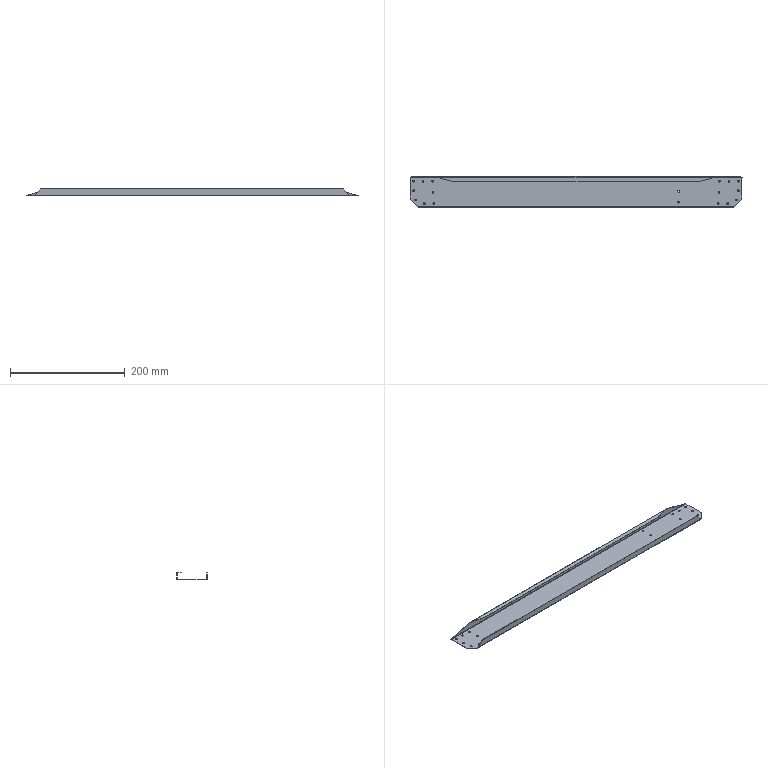Part | SolidWorks | features BaseBody 1 | 1 solid | 70 faces | box 579.6 x 52.529 x 13.429 mm | volume 22943 mm3 | cylinder 44 | plane 20 | spline 6 | commonest cylinder face diameters 3.2 x38 1.5 x3 2.5 x3